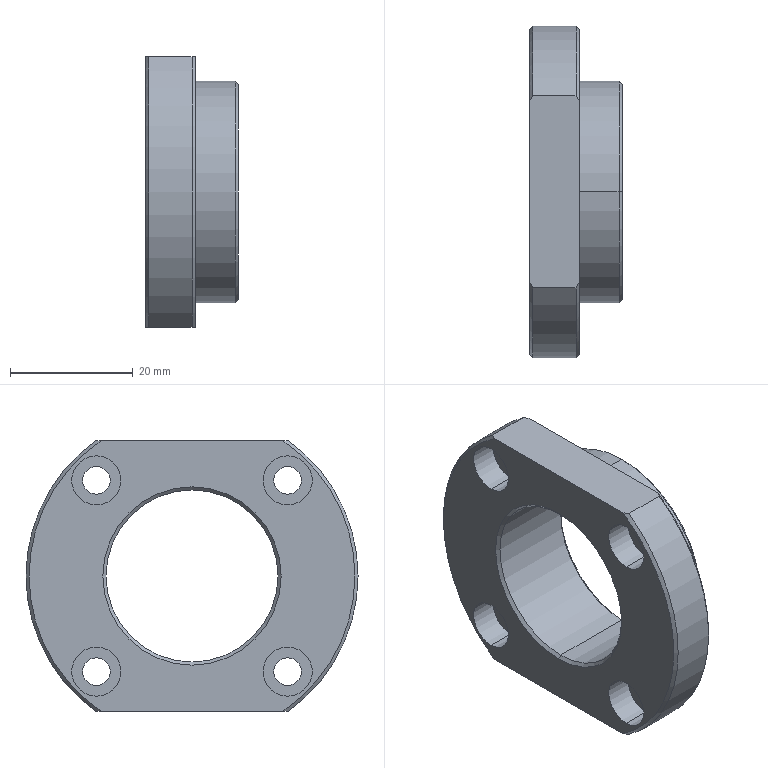Part | SolidWorks | features BaseBody 1 | 1 solid | 41 faces | box 15 x 54 x 44 mm | volume 13318 mm3 | cylinder 22 | cone 10 | plane 9 | commonest cylinder face diameters 4.5 x8 8 x8 28 x2 36 x2 54 x2
STEP:
#1=CARTESIAN_POINT('',(7.,0.,-14.));
#2=VERTEX_POINT('',#1);
#3=CARTESIAN_POINT('',(7.,-14.,0.));
#4=VERTEX_POINT('',#3);
#5=CARTESIAN_POINT('',(7.,0.,0.));
#6=DIRECTION('',(-1.,0.,0.));
#7=DIRECTION('',(0.,0.,1.));
#8=AXIS2_PLACEMENT_3D('',#5,#6,#7);
#9=CIRCLE('',#8,14.);
#10=EDGE_CURVE('',#2,#4,#9,.T.);
#11=ORIENTED_EDGE('',*,*,#10,.F.);
#12=CARTESIAN_POINT('',(-7.,0.,-14.));
#13=VERTEX_POINT('',#12);
#14=CARTESIAN_POINT('',(10.,0.,-14.));
#15=DIRECTION('',(-1.,0.,0.));
#16=VECTOR('',#15,1000.);
#17=LINE('',#14,#16);
#18=EDGE_CURVE('',#2,#13,#17,.T.);
#19=ORIENTED_EDGE('',*,*,#18,.T.);
#20=CARTESIAN_POINT('',(-7.,0.,14.));
#21=VERTEX_POINT('',#20);
#22=CARTESIAN_POINT('',(-7.,0.,0.));
#23=DIRECTION('',(1.,0.,0.));
#24=DIRECTION('',(0.,0.,1.));
#25=AXIS2_PLACEMENT_3D('',#22,#23,#24);
#26=CIRCLE('',#25,14.);
#27=EDGE_CURVE('',#21,#13,#26,.T.);
#28=ORIENTED_EDGE('',*,*,#27,.F.);
#29=CARTESIAN_POINT('',(7.,0.,14.));
#30=VERTEX_POINT('',#29);
#31=CARTESIAN_POINT('',(10.,0.,14.));
#32=DIRECTION('',(-1.,0.,0.));
#33=VECTOR('',#32,1000.);
#34=LINE('',#31,#33);
#35=EDGE_CURVE('',#30,#21,#34,.T.);
#36=ORIENTED_EDGE('',*,*,#35,.F.);
#37=CARTESIAN_POINT('',(7.,0.,0.));
#38=DIRECTION('',(-1.,0.,0.));
#39=DIRECTION('',(0.,0.,1.));
#40=AXIS2_PLACEMENT_3D('',#37,#38,#39);
#41=CIRCLE('',#40,14.);
#42=EDGE_CURVE('',#4,#30,#41,.T.);
#43=ORIENTED_EDGE('',*,*,#42,.F.);
#44=EDGE_LOOP('',(#11,#19,#28,#36,#43));
#45=FACE_OUTER_BOUND('',#44,.T.);
#46=CARTESIAN_POINT('',(10.,0.,0.));
#47=DIRECTION('',(-1.,0.,0.));
#48=DIRECTION('',(0.,0.,1.));
#49=AXIS2_PLACEMENT_3D('',#46,#47,#48);
#50=CYLINDRICAL_SURFACE('',#49,14.);
#51=ADVANCED_FACE('',(#45),#50,.F.);
#52=ORIENTED_EDGE('',*,*,#27,.T.);
#53=CARTESIAN_POINT('',(-7.5,0.,-14.5));
#54=VERTEX_POINT('',#53);
#55=CARTESIAN_POINT('',(-7.5,0.,-14.5));
#56=DIRECTION('',(-0.7071,0.,-0.7071));
#57=VECTOR('',#56,1000.);
#58=LINE('',#55,#57);
#59=EDGE_CURVE('',#13,#54,#58,.T.);
#60=ORIENTED_EDGE('',*,*,#59,.T.);
#61=CARTESIAN_POINT('',(-7.5,0.,14.5));
#62=VERTEX_POINT('',#61);
#63=CARTESIAN_POINT('',(-7.5,0.,0.));
#64=DIRECTION('',(1.,0.,0.));
#65=DIRECTION('',(0.,0.,1.));
#66=AXIS2_PLACEMENT_3D('',#63,#64,#65);
#67=CIRCLE('',#66,14.5);
#68=EDGE_CURVE('',#62,#54,#67,.T.);
#69=ORIENTED_EDGE('',*,*,#68,.F.);
#70=CARTESIAN_POINT('',(-7.5,0.,14.5));
#71=DIRECTION('',(-0.7071,0.,0.7071));
#72=VECTOR('',#71,1000.);
#73=LINE('',#70,#72);
#74=EDGE_CURVE('',#21,#62,#73,.T.);
#75=ORIENTED_EDGE('',*,*,#74,.F.);
#76=EDGE_LOOP('',(#52,#60,#69,#75));
#77=FACE_OUTER_BOUND('',#76,.T.);
#78=CARTESIAN_POINT('',(-7.5,0.,0.));
#79=DIRECTION('',(-1.,0.,0.));
#80=DIRECTION('',(0.,0.,1.));
#81=AXIS2_PLACEMENT_3D('',#78,#79,#80);
#82=CONICAL_SURFACE('',#81,14.5,0.7854);
#83=ADVANCED_FACE('',(#77),#82,.F.);
#84=CARTESIAN_POINT('',(7.,14.,0.));
#85=VERTEX_POINT('',#84);
#86=CARTESIAN_POINT('',(7.,0.,0.));
#87=DIRECTION('',(-1.,0.,0.));
#88=DIRECTION('',(0.,0.,1.));
#89=AXIS2_PLACEMENT_3D('',#86,#87,#88);
#90=CIRCLE('',#89,14.);
#91=EDGE_CURVE('',#85,#2,#90,.T.);
#92=ORIENTED_EDGE('',*,*,#91,.T.);
#93=ORIENTED_EDGE('',*,*,#10,.T.);
#94=CARTESIAN_POINT('',(7.5,-14.5,0.));
#95=VERTEX_POINT('',#94);
#96=CARTESIAN_POINT('',(7.5,-14.5,0.));
#97=DIRECTION('',(0.7071,-0.7071,0.));
#98=VECTOR('',#97,1000.);
#99=LINE('',#96,#98);
#100=EDGE_CURVE('',#4,#95,#99,.T.);
#101=ORIENTED_EDGE('',*,*,#100,.T.);
#102=CARTESIAN_POINT('',(7.5,14.5,0.));
#103=VERTEX_POINT('',#102);
#104=CARTESIAN_POINT('',(7.5,0.,0.));
#105=DIRECTION('',(-1.,0.,0.));
#106=DIRECTION('',(0.,1.,0.));
#107=AXIS2_PLACEMENT_3D('',#104,#105,#106);
#108=CIRCLE('',#107,14.5);
#109=EDGE_CURVE('',#103,#95,#108,.T.);
#110=ORIENTED_EDGE('',*,*,#109,.F.);
#111=CARTESIAN_POINT('',(7.5,14.5,0.));
#112=DIRECTION('',(0.7071,0.7071,0.));
#113=VECTOR('',#112,1000.);
#114=LINE('',#111,#113);
#115=EDGE_CURVE('',#85,#103,#114,.T.);
#116=ORIENTED_EDGE('',*,*,#115,.F.);
#117=EDGE_LOOP('',(#92,#93,#101,#110,#116));
#118=FACE_OUTER_BOUND('',#117,.T.);
#119=CARTESIAN_POINT('',(7.5,0.,0.));
#120=DIRECTION('',(1.,0.,0.));
#121=DIRECTION('',(0.,1.,0.));
#122=AXIS2_PLACEMENT_3D('',#119,#120,#121);
#123=CONICAL_SURFACE('',#122,14.5,0.7854);
#124=ADVANCED_FACE('',(#118),#123,.F.);
#125=CARTESIAN_POINT('',(-3.,15.556,11.556));
#126=VERTEX_POINT('',#125);
#127=CARTESIAN_POINT('',(-3.,15.556,19.556));
#128=VERTEX_POINT('',#127);
#129=CARTESIAN_POINT('',(-3.,15.556,15.556));
#130=DIRECTION('',(-1.,0.,0.));
#131=DIRECTION('',(0.,0.,1.));
#132=AXIS2_PLACEMENT_3D('',#129,#130,#131);
#133=CIRCLE('',#132,4.);
#134=EDGE_CURVE('',#126,#128,#133,.T.);
#135=ORIENTED_EDGE('',*,*,#134,.F.);
#136=CARTESIAN_POINT('',(-7.5,15.556,11.556));
#137=VERTEX_POINT('',#136);
#138=CARTESIAN_POINT('',(0.5,15.556,11.556));
#139=DIRECTION('',(-1.,0.,0.));
#140=VECTOR('',#139,1000.);
#141=LINE('',#138,#140);
#142=EDGE_CURVE('',#126,#137,#141,.T.);
#143=ORIENTED_EDGE('',*,*,#142,.T.);
#144=CARTESIAN_POINT('',(-7.5,15.556,19.556));
#145=VERTEX_POINT('',#144);
#146=CARTESIAN_POINT('',(-7.5,15.556,15.556));
#147=DIRECTION('',(1.,0.,0.));
#148=DIRECTION('',(0.,0.,1.));
#149=AXIS2_PLACEMENT_3D('',#146,#147,#148);
#150=CIRCLE('',#149,4.);
#151=EDGE_CURVE('',#145,#137,#150,.T.);
#152=ORIENTED_EDGE('',*,*,#151,.F.);
#153=CARTESIAN_POINT('',(0.5,15.556,19.556));
#154=DIRECTION('',(-1.,0.,0.));
#155=VECTOR('',#154,1000.);
#156=LINE('',#153,#155);
#157=EDGE_CURVE('',#128,#145,#156,.T.);
#158=ORIENTED_EDGE('',*,*,#157,.F.);
#159=EDGE_LOOP('',(#135,#143,#152,#158));
#160=FACE_OUTER_BOUND('',#159,.T.);
#161=CARTESIAN_POINT('',(0.5,15.556,15.556));
#162=DIRECTION('',(-1.,0.,0.));
#163=DIRECTION('',(0.,0.,1.));
#164=AXIS2_PLACEMENT_3D('',#161,#162,#163);
#165=CYLINDRICAL_SURFACE('',#164,4.);
#166=ADVANCED_FACE('',(#160),#165,.F.);
#167=CARTESIAN_POINT('',(-3.,-15.556,11.556));
#168=VERTEX_POINT('',#167);
#169=CARTESIAN_POINT('',(-3.,-15.556,19.556));
#170=VERTEX_POINT('',#169);
#171=CARTESIAN_POINT('',(-3.,-15.556,15.556));
#172=DIRECTION('',(-1.,0.,0.));
#173=DIRECTION('',(0.,0.,1.));
#174=AXIS2_PLACEMENT_3D('',#171,#172,#173);
#175=CIRCLE('',#174,4.);
#176=EDGE_CURVE('',#168,#170,#175,.T.);
#177=ORIENTED_EDGE('',*,*,#176,.F.);
#178=CARTESIAN_POINT('',(-7.5,-15.556,11.556));
#179=VERTEX_POINT('',#178);
#180=CARTESIAN_POINT('',(0.5,-15.556,11.556));
#181=DIRECTION('',(-1.,0.,0.));
#182=VECTOR('',#181,1000.);
#183=LINE('',#180,#182);
#184=EDGE_CURVE('',#168,#179,#183,.T.);
#185=ORIENTED_EDGE('',*,*,#184,.T.);
#186=CARTESIAN_POINT('',(-7.5,-15.556,19.556));
#187=VERTEX_POINT('',#186);
#188=CARTESIAN_POINT('',(-7.5,-15.556,15.556));
#189=DIRECTION('',(1.,0.,0.));
#190=DIRECTION('',(0.,0.,1.));
#191=AXIS2_PLACEMENT_3D('',#188,#189,#190);
#192=CIRCLE('',#191,4.);
#193=EDGE_CURVE('',#187,#179,#192,.T.);
#194=ORIENTED_EDGE('',*,*,#193,.F.);
#195=CARTESIAN_POINT('',(0.5,-15.556,19.556));
#196=DIRECTION('',(-1.,0.,0.));
#197=VECTOR('',#196,1000.);
#198=LINE('',#195,#197);
#199=EDGE_CURVE('',#170,#187,#198,.T.);
#200=ORIENTED_EDGE('',*,*,#199,.F.);
#201=EDGE_LOOP('',(#177,#185,#194,#200));
#202=FACE_OUTER_BOUND('',#201,.T.);
#203=CARTESIAN_POINT('',(0.5,-15.556,15.556));
#204=DIRECTION('',(-1.,0.,0.));
#205=DIRECTION('',(0.,0.,1.));
#206=AXIS2_PLACEMENT_3D('',#203,#204,#205);
#207=CYLINDRICAL_SURFACE('',#206,4.);
#208=ADVANCED_FACE('',(#202),#207,.F.);
#209=CARTESIAN_POINT('',(-3.,-15.556,-19.556));
#210=VERTEX_POINT('',#209);
#211=CARTESIAN_POINT('',(-3.,-15.556,-11.556));
#212=VERTEX_POINT('',#211);
#213=CARTESIAN_POINT('',(-3.,-15.556,-15.556));
#214=DIRECTION('',(-1.,0.,0.));
#215=DIRECTION('',(0.,0.,1.));
#216=AXIS2_PLACEMENT_3D('',#213,#214,#215);
#217=CIRCLE('',#216,4.);
#218=EDGE_CURVE('',#210,#212,#217,.T.);
#219=ORIENTED_EDGE('',*,*,#218,.F.);
#220=CARTESIAN_POINT('',(-7.5,-15.556,-19.556));
#221=VERTEX_POINT('',#220);
#222=CARTESIAN_POINT('',(0.5,-15.556,-19.556));
#223=DIRECTION('',(-1.,0.,0.));
#224=VECTOR('',#223,1000.);
#225=LINE('',#222,#224);
#226=EDGE_CURVE('',#210,#221,#225,.T.);
#227=ORIENTED_EDGE('',*,*,#226,.T.);
#228=CARTESIAN_POINT('',(-7.5,-15.556,-11.556));
#229=VERTEX_POINT('',#228);
#230=CARTESIAN_POINT('',(-7.5,-15.556,-15.556));
#231=DIRECTION('',(1.,0.,0.));
#232=DIRECTION('',(0.,0.,1.));
#233=AXIS2_PLACEMENT_3D('',#230,#231,#232);
#234=CIRCLE('',#233,4.);
#235=EDGE_CURVE('',#229,#221,#234,.T.);
#236=ORIENTED_EDGE('',*,*,#235,.F.);
#237=CARTESIAN_POINT('',(0.5,-15.556,-11.556));
#238=DIRECTION('',(-1.,0.,0.));
#239=VECTOR('',#238,1000.);
#240=LINE('',#237,#239);
#241=EDGE_CURVE('',#212,#229,#240,.T.);
#242=ORIENTED_EDGE('',*,*,#241,.F.);
#243=EDGE_LOOP('',(#219,#227,#236,#242));
#244=FACE_OUTER_BOUND('',#243,.T.);
#245=CARTESIAN_POINT('',(0.5,-15.556,-15.556));
#246=DIRECTION('',(-1.,0.,0.));
#247=DIRECTION('',(0.,0.,1.));
#248=AXIS2_PLACEMENT_3D('',#245,#246,#247);
#249=CYLINDRICAL_SURFACE('',#248,4.);
#250=ADVANCED_FACE('',(#244),#249,.F.);
#251=CARTESIAN_POINT('',(-3.,15.556,-19.556));
#252=VERTEX_POINT('',#251);
#253=CARTESIAN_POINT('',(-3.,15.556,-11.556));
#254=VERTEX_POINT('',#253);
#255=CARTESIAN_POINT('',(-3.,15.556,-15.556));
#256=DIRECTION('',(-1.,0.,0.));
#257=DIRECTION('',(0.,0.,1.));
#258=AXIS2_PLACEMENT_3D('',#255,#256,#257);
#259=CIRCLE('',#258,4.);
#260=EDGE_CURVE('',#252,#254,#259,.T.);
#261=ORIENTED_EDGE('',*,*,#260,.F.);
#262=CARTESIAN_POINT('',(-7.5,15.556,-19.556));
#263=VERTEX_POINT('',#262);
#264=CARTESIAN_POINT('',(0.5,15.556,-19.556));
#265=DIRECTION('',(-1.,0.,0.));
#266=VECTOR('',#265,1000.);
#267=LINE('',#264,#266);
#268=EDGE_CURVE('',#252,#263,#267,.T.);
#269=ORIENTED_EDGE('',*,*,#268,.T.);
#270=CARTESIAN_POINT('',(-7.5,15.556,-11.556));
#271=VERTEX_POINT('',#270);
#272=CARTESIAN_POINT('',(-7.5,15.556,-15.556));
#273=DIRECTION('',(1.,0.,0.));
#274=DIRECTION('',(0.,0.,1.));
#275=AXIS2_PLACEMENT_3D('',#272,#273,#274);
#276=CIRCLE('',#275,4.);
#277=EDGE_CURVE('',#271,#263,#276,.T.);
#278=ORIENTED_EDGE('',*,*,#277,.F.);
#279=CARTESIAN_POINT('',(0.5,15.556,-11.556));
#280=DIRECTION('',(-1.,0.,0.));
#281=VECTOR('',#280,1000.);
#282=LINE('',#279,#281);
#283=EDGE_CURVE('',#254,#271,#282,.T.);
#284=ORIENTED_EDGE('',*,*,#283,.F.);
#285=EDGE_LOOP('',(#261,#269,#278,#284));
#286=FACE_OUTER_BOUND('',#285,.T.);
#287=CARTESIAN_POINT('',(0.5,15.556,-15.556));
#288=DIRECTION('',(-1.,0.,0.));
#289=DIRECTION('',(0.,0.,1.));
#290=AXIS2_PLACEMENT_3D('',#287,#288,#289);
#291=CYLINDRICAL_SURFACE('',#290,4.);
#292=ADVANCED_FACE('',(#286),#291,.F.);
#293=CARTESIAN_POINT('',(7.5,0.,-17.5));
#294=VERTEX_POINT('',#293);
#295=CARTESIAN_POINT('',(7.5,0.,17.5));
#296=VERTEX_POINT('',#295);
#297=CARTESIAN_POINT('',(7.5,0.,0.));
#298=DIRECTION('',(1.,0.,0.));
#299=DIRECTION('',(0.,0.,1.));
#300=AXIS2_PLACEMENT_3D('',#297,#298,#299);
#301=CIRCLE('',#300,17.5);
#302=EDGE_CURVE('',#294,#296,#301,.T.);
#303=ORIENTED_EDGE('',*,*,#302,.F.);
#304=CARTESIAN_POINT('',(7.,0.,-18.));
#305=VERTEX_POINT('',#304);
#306=CARTESIAN_POINT('',(7.,0.,-18.));
#307=DIRECTION('',(-0.7071,0.,-0.7071));
#308=VECTOR('',#307,1000.);
#309=LINE('',#306,#308);
#310=EDGE_CURVE('',#294,#305,#309,.T.);
#311=ORIENTED_EDGE('',*,*,#310,.T.);
#312=CARTESIAN_POINT('',(7.,0.,18.));
#313=VERTEX_POINT('',#312);
#314=CARTESIAN_POINT('',(7.,0.,0.));
#315=DIRECTION('',(1.,0.,0.));
#316=DIRECTION('',(0.,0.,1.));
#317=AXIS2_PLACEMENT_3D('',#314,#315,#316);
#318=CIRCLE('',#317,18.);
#319=EDGE_CURVE('',#305,#313,#318,.T.);
#320=ORIENTED_EDGE('',*,*,#319,.T.);
#321=CARTESIAN_POINT('',(7.,0.,18.));
#322=DIRECTION('',(-0.7071,0.,0.7071));
#323=VECTOR('',#322,1000.);
#324=LINE('',#321,#323);
#325=EDGE_CURVE('',#296,#313,#324,.T.);
#326=ORIENTED_EDGE('',*,*,#325,.F.);
#327=EDGE_LOOP('',(#303,#311,#320,#326));
#328=FACE_OUTER_BOUND('',#327,.T.);
#329=CARTESIAN_POINT('',(7.,0.,0.));
#330=DIRECTION('',(-1.,0.,0.));
#331=DIRECTION('',(0.,0.,1.));
#332=AXIS2_PLACEMENT_3D('',#329,#330,#331);
#333=CONICAL_SURFACE('',#332,18.,0.7854);
#334=ADVANCED_FACE('',(#328),#333,.T.);
#335=ORIENTED_EDGE('',*,*,#319,.F.);
#336=CARTESIAN_POINT('',(0.5,0.,-18.));
#337=VERTEX_POINT('',#336);
#338=CARTESIAN_POINT('',(10.,0.,-18.));
#339=DIRECTION('',(-1.,0.,0.));
#340=VECTOR('',#339,1000.);
#341=LINE('',#338,#340);
#342=EDGE_CURVE('',#305,#337,#341,.T.);
#343=ORIENTED_EDGE('',*,*,#342,.T.);
#344=CARTESIAN_POINT('',(0.5,0.,18.));
#345=VERTEX_POINT('',#344);
#346=CARTESIAN_POINT('',(0.5,0.,0.));
#347=DIRECTION('',(-1.,0.,0.));
#348=DIRECTION('',(0.,0.,1.));
#349=AXIS2_PLACEMENT_3D('',#346,#347,#348);
#350=CIRCLE('',#349,18.);
#351=EDGE_CURVE('',#345,#337,#350,.T.);
#352=ORIENTED_EDGE('',*,*,#351,.F.);
#353=CARTESIAN_POINT('',(10.,0.,18.));
#354=DIRECTION('',(-1.,0.,0.));
#355=VECTOR('',#354,1000.);
#356=LINE('',#353,#355);
#357=EDGE_CURVE('',#313,#345,#356,.T.);
#358=ORIENTED_EDGE('',*,*,#357,.F.);
#359=EDGE_LOOP('',(#335,#343,#352,#358));
#360=FACE_OUTER_BOUND('',#359,.T.);
#361=CARTESIAN_POINT('',(10.,0.,0.));
#362=DIRECTION('',(-1.,0.,0.));
#363=DIRECTION('',(0.,0.,1.));
#364=AXIS2_PLACEMENT_3D('',#361,#362,#363);
#365=CYLINDRICAL_SURFACE('',#364,18.);
#366=ADVANCED_FACE('',(#360),#365,.T.);
#367=CARTESIAN_POINT('',(0.5,15.556,13.306));
#368=VERTEX_POINT('',#367);
#369=CARTESIAN_POINT('',(0.5,15.556,17.806));
#370=VERTEX_POINT('',#369);
#371=CARTESIAN_POINT('',(0.5,15.556,15.556));
#372=DIRECTION('',(-1.,0.,0.));
#373=DIRECTION('',(0.,0.,1.));
#374=AXIS2_PLACEMENT_3D('',#371,#372,#373);
#375=CIRCLE('',#374,2.25);
#376=EDGE_CURVE('',#368,#370,#375,.T.);
#377=ORIENTED_EDGE('',*,*,#376,.F.);
#378=CARTESIAN_POINT('',(-3.,15.556,13.306));
#379=VERTEX_POINT('',#378);
#380=CARTESIAN_POINT('',(0.5,15.556,13.306));
#381=DIRECTION('',(-1.,0.,0.));
#382=VECTOR('',#381,1000.);
#383=LINE('',#380,#382);
#384=EDGE_CURVE('',#368,#379,#383,.T.);
#385=ORIENTED_EDGE('',*,*,#384,.T.);
#386=CARTESIAN_POINT('',(-3.,15.556,17.806));
#387=VERTEX_POINT('',#386);
#388=CARTESIAN_POINT('',(-3.,15.556,15.556));
#389=DIRECTION('',(1.,0.,0.));
#390=DIRECTION('',(0.,0.,1.));
#391=AXIS2_PLACEMENT_3D('',#388,#389,#390);
#392=CIRCLE('',#391,2.25);
#393=EDGE_CURVE('',#387,#379,#392,.T.);
#394=ORIENTED_EDGE('',*,*,#393,.F.);
#395=CARTESIAN_POINT('',(0.5,15.556,17.806));
#396=DIRECTION('',(-1.,0.,0.));
#397=VECTOR('',#396,1000.);
#398=LINE('',#395,#397);
#399=EDGE_CURVE('',#370,#387,#398,.T.);
#400=ORIENTED_EDGE('',*,*,#399,.F.);
#401=EDGE_LOOP('',(#377,#385,#394,#400));
#402=FACE_OUTER_BOUND('',#401,.T.);
#403=CARTESIAN_POINT('',(0.5,15.556,15.556));
#404=DIRECTION('',(-1.,0.,0.));
#405=DIRECTION('',(0.,0.,1.));
#406=AXIS2_PLACEMENT_3D('',#403,#404,#405);
#407=CYLINDRICAL_SURFACE('',#406,2.25);
#408=ADVANCED_FACE('',(#402),#407,.F.);
#409=CARTESIAN_POINT('',(0.5,-15.556,13.306));
#410=VERTEX_POINT('',#409);
#411=CARTESIAN_POINT('',(0.5,-15.556,17.806));
#412=VERTEX_POINT('',#411);
#413=CARTESIAN_POINT('',(0.5,-15.556,15.556));
#414=DIRECTION('',(-1.,0.,0.));
#415=DIRECTION('',(0.,0.,1.));
#416=AXIS2_PLACEMENT_3D('',#413,#414,#415);
#417=CIRCLE('',#416,2.25);
#418=EDGE_CURVE('',#410,#412,#417,.T.);
#419=ORIENTED_EDGE('',*,*,#418,.F.);
#420=CARTESIAN_POINT('',(-3.,-15.556,13.306));
#421=VERTEX_POINT('',#420);
#422=CARTESIAN_POINT('',(0.5,-15.556,13.306));
#423=DIRECTION('',(-1.,0.,0.));
#424=VECTOR('',#423,1000.);
#425=LINE('',#422,#424);
#426=EDGE_CURVE('',#410,#421,#425,.T.);
#427=ORIENTED_EDGE('',*,*,#426,.T.);
#428=CARTESIAN_POINT('',(-3.,-15.556,17.806));
#429=VERTEX_POINT('',#428);
#430=CARTESIAN_POINT('',(-3.,-15.556,15.556));
#431=DIRECTION('',(1.,0.,0.));
#432=DIRECTION('',(0.,0.,1.));
#433=AXIS2_PLACEMENT_3D('',#430,#431,#432);
#434=CIRCLE('',#433,2.25);
#435=EDGE_CURVE('',#429,#421,#434,.T.);
#436=ORIENTED_EDGE('',*,*,#435,.F.);
#437=CARTESIAN_POINT('',(0.5,-15.556,17.806));
#438=DIRECTION('',(-1.,0.,0.));
#439=VECTOR('',#438,1000.);
#440=LINE('',#437,#439);
#441=EDGE_CURVE('',#412,#429,#440,.T.);
#442=ORIENTED_EDGE('',*,*,#441,.F.);
#443=EDGE_LOOP('',(#419,#427,#436,#442));
#444=FACE_OUTER_BOUND('',#443,.T.);
#445=CARTESIAN_POINT('',(0.5,-15.556,15.556));
#446=DIRECTION('',(-1.,0.,0.));
#447=DIRECTION('',(0.,0.,1.));
#448=AXIS2_PLACEMENT_3D('',#445,#446,#447);
#449=CYLINDRICAL_SURFACE('',#448,2.25);
#450=ADVANCED_FACE('',(#444),#449,.F.);
#451=CARTESIAN_POINT('',(0.5,-15.556,-17.806));
#452=VERTEX_POINT('',#451);
#453=CARTESIAN_POINT('',(0.5,-15.556,-13.306));
#454=VERTEX_POINT('',#453);
#455=CARTESIAN_POINT('',(0.5,-15.556,-15.556));
#456=DIRECTION('',(-1.,0.,0.));
#457=DIRECTION('',(0.,0.,1.));
#458=AXIS2_PLACEMENT_3D('',#455,#456,#457);
#459=CIRCLE('',#458,2.25);
#460=EDGE_CURVE('',#452,#454,#459,.T.);
#461=ORIENTED_EDGE('',*,*,#460,.F.);
#462=CARTESIAN_POINT('',(-3.,-15.556,-17.806));
#463=VERTEX_POINT('',#462);
#464=CARTESIAN_POINT('',(0.5,-15.556,-17.806));
#465=DIRECTION('',(-1.,0.,0.));
#466=VECTOR('',#465,1000.);
#467=LINE('',#464,#466);
#468=EDGE_CURVE('',#452,#463,#467,.T.);
#469=ORIENTED_EDGE('',*,*,#468,.T.);
#470=CARTESIAN_POINT('',(-3.,-15.556,-13.306));
#471=VERTEX_POINT('',#470);
#472=CARTESIAN_POINT('',(-3.,-15.556,-15.556));
#473=DIRECTION('',(1.,0.,0.));
#474=DIRECTION('',(0.,0.,1.));
#475=AXIS2_PLACEMENT_3D('',#472,#473,#474);
#476=CIRCLE('',#475,2.25);
#477=EDGE_CURVE('',#471,#463,#476,.T.);
#478=ORIENTED_EDGE('',*,*,#477,.F.);
#479=CARTESIAN_POINT('',(0.5,-15.556,-13.306));
#480=DIRECTION('',(-1.,0.,0.));
#481=VECTOR('',#480,1000.);
#482=LINE('',#479,#481);
#483=EDGE_CURVE('',#454,#471,#482,.T.);
#484=ORIENTED_EDGE('',*,*,#483,.F.);
#485=EDGE_LOOP('',(#461,#469,#478,#484));
#486=FACE_OUTER_BOUND('',#485,.T.);
#487=CARTESIAN_POINT('',(0.5,-15.556,-15.556));
#488=DIRECTION('',(-1.,0.,0.));
#489=DIRECTION('',(0.,0.,1.));
#490=AXIS2_PLACEMENT_3D('',#487,#488,#489);
#491=CYLINDRICAL_SURFACE('',#490,2.25);
#492=ADVANCED_FACE('',(#486),#491,.F.);
#493=CARTESIAN_POINT('',(0.5,15.556,-17.806));
#494=VERTEX_POINT('',#493);
#495=CARTESIAN_POINT('',(0.5,15.556,-13.306));
#496=VERTEX_POINT('',#495);
#497=CARTESIAN_POINT('',(0.5,15.556,-15.556));
#498=DIRECTION('',(-1.,0.,0.));
#499=DIRECTION('',(0.,0.,1.));
#500=AXIS2_PLACEMENT_3D('',#497,#498,#499);
#501=CIRCLE('',#500,2.25);
#502=EDGE_CURVE('',#494,#496,#501,.T.);
#503=ORIENTED_EDGE('',*,*,#502,.F.);
#504=CARTESIAN_POINT('',(-3.,15.556,-17.806));
#505=VERTEX_POINT('',#504);
#506=CARTESIAN_POINT('',(0.5,15.556,-17.806));
#507=DIRECTION('',(-1.,0.,0.));
#508=VECTOR('',#507,1000.);
#509=LINE('',#506,#508);
#510=EDGE_CURVE('',#494,#505,#509,.T.);
#511=ORIENTED_EDGE('',*,*,#510,.T.);
#512=CARTESIAN_POINT('',(-3.,15.556,-13.306));
#513=VERTEX_POINT('',#512);
#514=CARTESIAN_POINT('',(-3.,15.556,-15.556));
#515=DIRECTION('',(1.,0.,0.));
#516=DIRECTION('',(0.,0.,1.));
#517=AXIS2_PLACEMENT_3D('',#514,#515,#516);
#518=CIRCLE('',#517,2.25);
#519=EDGE_CURVE('',#513,#505,#518,.T.);
#520=ORIENTED_EDGE('',*,*,#519,.F.);
#521=CARTESIAN_POINT('',(0.5,15.556,-13.306));
#522=DIRECTION('',(-1.,0.,0.));
#523=VECTOR('',#522,1000.);
#524=LINE('',#521,#523);
#525=EDGE_CURVE('',#496,#513,#524,.T.);
#526=ORIENTED_EDGE('',*,*,#525,.F.);
#527=EDGE_LOOP('',(#503,#511,#520,#526));
#528=FACE_OUTER_BOUND('',#527,.T.);
#529=CARTESIAN_POINT('',(0.5,15.556,-15.556));
#530=DIRECTION('',(-1.,0.,0.));
#531=DIRECTION('',(0.,0.,1.));
#532=AXIS2_PLACEMENT_3D('',#529,#530,#531);
#533=CYLINDRICAL_SURFACE('',#532,2.25);
#534=ADVANCED_FACE('',(#528),#533,.F.);
#535=ORIENTED_EDGE('',*,*,#18,.F.);
#536=ORIENTED_EDGE('',*,*,#91,.F.);
#537=CARTESIAN_POINT('',(7.,0.,0.));
#538=DIRECTION('',(-1.,0.,0.));
#539=DIRECTION('',(0.,0.,1.));
#540=AXIS2_PLACEMENT_3D('',#537,#538,#539);
#541=CIRCLE('',#540,14.);
#542=EDGE_CURVE('',#30,#85,#541,.T.);
#543=ORIENTED_EDGE('',*,*,#542,.F.);
#544=ORIENTED_EDGE('',*,*,#35,.T.);
#545=CARTESIAN_POINT('',(-7.,0.,0.));
#546=DIRECTION('',(1.,0.,0.));
#547=DIRECTION('',(0.,0.,1.));
#548=AXIS2_PLACEMENT_3D('',#545,#546,#547);
#549=CIRCLE('',#548,14.);
#550=EDGE_CURVE('',#13,#21,#549,.T.);
#551=ORIENTED_EDGE('',*,*,#550,.F.);
#552=EDGE_LOOP('',(#535,#536,#543,#544,#551));
#553=FACE_OUTER_BOUND('',#552,.T.);
#554=CARTESIAN_POINT('',(10.,0.,0.));
#555=DIRECTION('',(-1.,0.,0.));
#556=DIRECTION('',(0.,0.,1.));
#557=AXIS2_PLACEMENT_3D('',#554,#555,#556);
#558=CYLINDRICAL_SURFACE('',#557,14.);
#559=ADVANCED_FACE('',(#553),#558,.F.);
#560=ORIENTED_EDGE('',*,*,#59,.F.);
#561=ORIENTED_EDGE('',*,*,#550,.T.);
#562=ORIENTED_EDGE('',*,*,#74,.T.);
#563=CARTESIAN_POINT('',(-7.5,0.,0.));
#564=DIRECTION('',(1.,0.,0.));
#565=DIRECTION('',(0.,0.,1.));
#566=AXIS2_PLACEMENT_3D('',#563,#564,#565);
#567=CIRCLE('',#566,14.5);
#568=EDGE_CURVE('',#54,#62,#567,.T.);
#569=ORIENTED_EDGE('',*,*,#568,.F.);
#570=EDGE_LOOP('',(#560,#561,#562,#569));
#571=FACE_OUTER_BOUND('',#570,.T.);
#572=CARTESIAN_POINT('',(-7.5,0.,0.));
#573=DIRECTION('',(-1.,0.,0.));
#574=DIRECTION('',(0.,0.,1.));
#575=AXIS2_PLACEMENT_3D('',#572,#573,#574);
#576=CONICAL_SURFACE('',#575,14.5,0.7854);
#577=ADVANCED_FACE('',(#571),#576,.F.);
#578=ORIENTED_EDGE('',*,*,#100,.F.);
#579=ORIENTED_EDGE('',*,*,#42,.T.);
#580=ORIENTED_EDGE('',*,*,#542,.T.);
#581=ORIENTED_EDGE('',*,*,#115,.T.);
#582=CARTESIAN_POINT('',(7.5,0.,0.));
#583=DIRECTION('',(-1.,0.,0.));
#584=DIRECTION('',(0.,1.,0.));
#585=AXIS2_PLACEMENT_3D('',#582,#583,#584);
#586=CIRCLE('',#585,14.5);
#587=EDGE_CURVE('',#95,#103,#586,.T.);
#588=ORIENTED_EDGE('',*,*,#587,.F.);
#589=EDGE_LOOP('',(#578,#579,#580,#581,#588));
#590=FACE_OUTER_BOUND('',#589,.T.);
#591=CARTESIAN_POINT('',(7.5,0.,0.));
#592=DIRECTION('',(1.,0.,0.));
#593=DIRECTION('',(0.,1.,0.));
#594=AXIS2_PLACEMENT_3D('',#591,#592,#593);
#595=CONICAL_SURFACE('',#594,14.5,0.7854);
#596=ADVANCED_FACE('',(#590),#595,.F.);
#597=ORIENTED_EDGE('',*,*,#151,.T.);
#598=CARTESIAN_POINT('',(-7.5,15.556,15.556));
#599=DIRECTION('',(1.,0.,0.));
#600=DIRECTION('',(0.,0.,1.));
#601=AXIS2_PLACEMENT_3D('',#598,#599,#600);
#602=CIRCLE('',#601,4.);
#603=EDGE_CURVE('',#137,#145,#602,.T.);
#604=ORIENTED_EDGE('',*,*,#603,.T.);
#605=EDGE_LOOP('',(#597,#604));
#606=FACE_BOUND('',#605,.T.);
#607=ORIENTED_EDGE('',*,*,#193,.T.);
#608=CARTESIAN_POINT('',(-7.5,-15.556,15.556));
#609=DIRECTION('',(1.,0.,0.));
#610=DIRECTION('',(0.,0.,1.));
#611=AXIS2_PLACEMENT_3D('',#608,#609,#610);
#612=CIRCLE('',#611,4.);
#613=EDGE_CURVE('',#179,#187,#612,.T.);
#614=ORIENTED_EDGE('',*,*,#613,.T.);
#615=EDGE_LOOP('',(#607,#614));
#616=FACE_BOUND('',#615,.T.);
#617=ORIENTED_EDGE('',*,*,#235,.T.);
#618=CARTESIAN_POINT('',(-7.5,-15.556,-15.556));
#619=DIRECTION('',(1.,0.,0.));
#620=DIRECTION('',(0.,0.,1.));
#621=AXIS2_PLACEMENT_3D('',#618,#619,#620);
#622=CIRCLE('',#621,4.);
#623=EDGE_CURVE('',#221,#229,#622,.T.);
#624=ORIENTED_EDGE('',*,*,#623,.T.);
#625=EDGE_LOOP('',(#617,#624));
#626=FACE_BOUND('',#625,.T.);
#627=ORIENTED_EDGE('',*,*,#277,.T.);
#628=CARTESIAN_POINT('',(-7.5,15.556,-15.556));
#629=DIRECTION('',(1.,0.,0.));
#630=DIRECTION('',(0.,0.,1.));
#631=AXIS2_PLACEMENT_3D('',#628,#629,#630);
#632=CIRCLE('',#631,4.);
#633=EDGE_CURVE('',#263,#271,#632,.T.);
#634=ORIENTED_EDGE('',*,*,#633,.T.);
#635=EDGE_LOOP('',(#627,#634));
#636=FACE_BOUND('',#635,.T.);
#637=CARTESIAN_POINT('',(-7.5,-14.773,22.));
#638=VERTEX_POINT('',#637);
#639=CARTESIAN_POINT('',(-7.5,14.773,22.));
#640=VERTEX_POINT('',#639);
#641=CARTESIAN_POINT('',(-7.5,26.5,22.));
#642=DIRECTION('',(0.,1.,0.));
#643=VECTOR('',#642,1000.);
#644=LINE('',#641,#643);
#645=EDGE_CURVE('',#638,#640,#644,.T.);
#646=ORIENTED_EDGE('',*,*,#645,.T.);
#647=CARTESIAN_POINT('',(-7.5,14.773,-22.));
#648=VERTEX_POINT('',#647);
#649=CARTESIAN_POINT('',(-7.5,0.,0.));
#650=DIRECTION('',(-1.,0.,0.));
#651=DIRECTION('',(0.,0.,-1.));
#652=AXIS2_PLACEMENT_3D('',#649,#650,#651);
#653=CIRCLE('',#652,26.5);
#654=EDGE_CURVE('',#640,#648,#653,.T.);
#655=ORIENTED_EDGE('',*,*,#654,.T.);
#656=CARTESIAN_POINT('',(-7.5,-14.773,-22.));
#657=VERTEX_POINT('',#656);
#658=CARTESIAN_POINT('',(-7.5,26.5,-22.));
#659=DIRECTION('',(0.,-1.,0.));
#660=VECTOR('',#659,1000.);
#661=LINE('',#658,#660);
#662=EDGE_CURVE('',#648,#657,#661,.T.);
#663=ORIENTED_EDGE('',*,*,#662,.T.);
#664=CARTESIAN_POINT('',(-7.5,0.,0.));
#665=DIRECTION('',(-1.,0.,0.));
#666=DIRECTION('',(0.,0.,-1.));
#667=AXIS2_PLACEMENT_3D('',#664,#665,#666);
#668=CIRCLE('',#667,26.5);
#669=EDGE_CURVE('',#657,#638,#668,.T.);
#670=ORIENTED_EDGE('',*,*,#669,.T.);
#671=EDGE_LOOP('',(#646,#655,#663,#670));
#672=FACE_OUTER_BOUND('',#671,.T.);
#673=ORIENTED_EDGE('',*,*,#68,.T.);
#674=ORIENTED_EDGE('',*,*,#568,.T.);
#675=EDGE_LOOP('',(#673,#674));
#676=FACE_BOUND('',#675,.T.);
#677=CARTESIAN_POINT('',(-7.5,26.5,0.));
#678=DIRECTION('',(-1.,0.,0.));
#679=DIRECTION('',(0.,0.,1.));
#680=AXIS2_PLACEMENT_3D('',#677,#678,#679);
#681=PLANE('',#680);
#682=ADVANCED_FACE('',(#606,#616,#626,#636,#672,#676),#681,.T.);
#683=ORIENTED_EDGE('',*,*,#109,.T.);
#684=ORIENTED_EDGE('',*,*,#587,.T.);
#685=EDGE_LOOP('',(#683,#684));
#686=FACE_BOUND('',#685,.T.);
#687=CARTESIAN_POINT('',(7.5,0.,0.));
#688=DIRECTION('',(1.,0.,0.));
#689=DIRECTION('',(0.,0.,1.));
#690=AXIS2_PLACEMENT_3D('',#687,#688,#689);
#691=CIRCLE('',#690,17.5);
#692=EDGE_CURVE('',#296,#294,#691,.T.);
#693=ORIENTED_EDGE('',*,*,#692,.T.);
#694=ORIENTED_EDGE('',*,*,#302,.T.);
#695=EDGE_LOOP('',(#693,#694));
#696=FACE_OUTER_BOUND('',#695,.T.);
#697=CARTESIAN_POINT('',(7.5,14.5,0.));
#698=DIRECTION('',(1.,0.,0.));
#699=DIRECTION('',(0.,0.,-1.));
#700=AXIS2_PLACEMENT_3D('',#697,#698,#699);
#701=PLANE('',#700);
#702=ADVANCED_FACE('',(#686,#696),#701,.T.);
#703=ORIENTED_EDGE('',*,*,#142,.F.);
#704=CARTESIAN_POINT('',(-3.,15.556,15.556));
#705=DIRECTION('',(-1.,0.,0.));
#706=DIRECTION('',(0.,0.,1.));
#707=AXIS2_PLACEMENT_3D('',#704,#705,#706);
#708=CIRCLE('',#707,4.);
#709=EDGE_CURVE('',#128,#126,#708,.T.);
#710=ORIENTED_EDGE('',*,*,#709,.F.);
#711=ORIENTED_EDGE('',*,*,#157,.T.);
#712=ORIENTED_EDGE('',*,*,#603,.F.);
#713=EDGE_LOOP('',(#703,#710,#711,#712));
#714=FACE_OUTER_BOUND('',#713,.T.);
#715=CARTESIAN_POINT('',(0.5,15.556,15.556));
#716=DIRECTION('',(-1.,0.,0.));
#717=DIRECTION('',(0.,0.,1.));
#718=AXIS2_PLACEMENT_3D('',#715,#716,#717);
#719=CYLINDRICAL_SURFACE('',#718,4.);
#720=ADVANCED_FACE('',(#714),#719,.F.);
#721=ORIENTED_EDGE('',*,*,#184,.F.);
#722=CARTESIAN_POINT('',(-3.,-15.556,15.556));
#723=DIRECTION('',(-1.,0.,0.));
#724=DIRECTION('',(0.,0.,1.));
#725=AXIS2_PLACEMENT_3D('',#722,#723,#724);
#726=CIRCLE('',#725,4.);
#727=EDGE_CURVE('',#170,#168,#726,.T.);
#728=ORIENTED_EDGE('',*,*,#727,.F.);
#729=ORIENTED_EDGE('',*,*,#199,.T.);
#730=ORIENTED_EDGE('',*,*,#613,.F.);
#731=EDGE_LOOP('',(#721,#728,#729,#730));
#732=FACE_OUTER_BOUND('',#731,.T.);
#733=CARTESIAN_POINT('',(0.5,-15.556,15.556));
#734=DIRECTION('',(-1.,0.,0.));
#735=DIRECTION('',(0.,0.,1.));
#736=AXIS2_PLACEMENT_3D('',#733,#734,#735);
#737=CYLINDRICAL_SURFACE('',#736,4.);
#738=ADVANCED_FACE('',(#732),#737,.F.);
#739=ORIENTED_EDGE('',*,*,#226,.F.);
#740=CARTESIAN_POINT('',(-3.,-15.556,-15.556));
#741=DIRECTION('',(-1.,0.,0.));
#742=DIRECTION('',(0.,0.,1.));
#743=AXIS2_PLACEMENT_3D('',#740,#741,#742);
#744=CIRCLE('',#743,4.);
#745=EDGE_CURVE('',#212,#210,#744,.T.);
#746=ORIENTED_EDGE('',*,*,#745,.F.);
#747=ORIENTED_EDGE('',*,*,#241,.T.);
#748=ORIENTED_EDGE('',*,*,#623,.F.);
#749=EDGE_LOOP('',(#739,#746,#747,#748));
#750=FACE_OUTER_BOUND('',#749,.T.);
#751=CARTESIAN_POINT('',(0.5,-15.556,-15.556));
#752=DIRECTION('',(-1.,0.,0.));
#753=DIRECTION('',(0.,0.,1.));
#754=AXIS2_PLACEMENT_3D('',#751,#752,#753);
#755=CYLINDRICAL_SURFACE('',#754,4.);
#756=ADVANCED_FACE('',(#750),#755,.F.);
#757=ORIENTED_EDGE('',*,*,#268,.F.);
#758=CARTESIAN_POINT('',(-3.,15.556,-15.556));
#759=DIRECTION('',(-1.,0.,0.));
#760=DIRECTION('',(0.,0.,1.));
#761=AXIS2_PLACEMENT_3D('',#758,#759,#760);
#762=CIRCLE('',#761,4.);
#763=EDGE_CURVE('',#254,#252,#762,.T.);
#764=ORIENTED_EDGE('',*,*,#763,.F.);
#765=ORIENTED_EDGE('',*,*,#283,.T.);
#766=ORIENTED_EDGE('',*,*,#633,.F.);
#767=EDGE_LOOP('',(#757,#764,#765,#766));
#768=FACE_OUTER_BOUND('',#767,.T.);
#769=CARTESIAN_POINT('',(0.5,15.556,-15.556));
#770=DIRECTION('',(-1.,0.,0.));
#771=DIRECTION('',(0.,0.,1.));
#772=AXIS2_PLACEMENT_3D('',#769,#770,#771);
#773=CYLINDRICAL_SURFACE('',#772,4.);
#774=ADVANCED_FACE('',(#768),#773,.F.);
#775=CARTESIAN_POINT('',(-7.,15.652,22.));
#776=VERTEX_POINT('',#775);
#777=CARTESIAN_POINT('',(-7.5,14.773,22.));
#778=CARTESIAN_POINT('',(-7.336,15.068,22.));
#779=CARTESIAN_POINT('',(-7.169,15.361,22.));
#780=CARTESIAN_POINT('',(-7.,15.652,22.));
#781=B_SPLINE_CURVE_WITH_KNOTS('',3,(#777,#778,#779,#780),.UNSPECIFIED.,.F.,.F.,(4,4),(0.,0.001011),.UNSPECIFIED.);
#782=EDGE_CURVE('',#640,#776,#781,.T.);
#783=ORIENTED_EDGE('',*,*,#782,.T.);
#784=CARTESIAN_POINT('',(-7.,15.652,-22.));
#785=VERTEX_POINT('',#784);
#786=CARTESIAN_POINT('',(-7.,0.,0.));
#787=DIRECTION('',(-1.,0.,0.));
#788=DIRECTION('',(0.,0.,-1.));
#789=AXIS2_PLACEMENT_3D('',#786,#787,#788);
#790=CIRCLE('',#789,27.);
#791=EDGE_CURVE('',#776,#785,#790,.T.);
#792=ORIENTED_EDGE('',*,*,#791,.T.);
#793=CARTESIAN_POINT('',(-7.,15.652,-22.));
#794=CARTESIAN_POINT('',(-7.169,15.361,-22.));
#795=CARTESIAN_POINT('',(-7.336,15.068,-22.));
#796=CARTESIAN_POINT('',(-7.5,14.773,-22.));
#797=B_SPLINE_CURVE_WITH_KNOTS('',3,(#793,#794,#795,#796),.UNSPECIFIED.,.F.,.F.,(4,4),(0.,0.001011),.UNSPECIFIED.);
#798=EDGE_CURVE('',#785,#648,#797,.T.);
#799=ORIENTED_EDGE('',*,*,#798,.T.);
#800=ORIENTED_EDGE('',*,*,#654,.F.);
#801=EDGE_LOOP('',(#783,#792,#799,#800));
#802=FACE_OUTER_BOUND('',#801,.T.);
#803=CARTESIAN_POINT('',(-7.,0.,0.));
#804=DIRECTION('',(1.,0.,0.));
#805=DIRECTION('',(0.,0.,-1.));
#806=AXIS2_PLACEMENT_3D('',#803,#804,#805);
#807=CONICAL_SURFACE('',#806,27.,0.7854);
#808=ADVANCED_FACE('',(#802),#807,.T.);
#809=CARTESIAN_POINT('',(0.,15.652,22.));
#810=VERTEX_POINT('',#809);
#811=CARTESIAN_POINT('',(0.5,15.652,22.));
#812=DIRECTION('',(1.,0.,0.));
#813=VECTOR('',#812,1000.);
#814=LINE('',#811,#813);
#815=EDGE_CURVE('',#776,#810,#814,.T.);
#816=ORIENTED_EDGE('',*,*,#815,.F.);
#817=ORIENTED_EDGE('',*,*,#782,.F.);
#818=ORIENTED_EDGE('',*,*,#645,.F.);
#819=CARTESIAN_POINT('',(-7.,-15.652,22.));
#820=VERTEX_POINT('',#819);
#821=CARTESIAN_POINT('',(-7.,-15.652,22.));
#822=CARTESIAN_POINT('',(-7.169,-15.361,22.));
#823=CARTESIAN_POINT('',(-7.336,-15.068,22.));
#824=CARTESIAN_POINT('',(-7.5,-14.773,22.));
#825=B_SPLINE_CURVE_WITH_KNOTS('',3,(#821,#822,#823,#824),.UNSPECIFIED.,.F.,.F.,(4,4),(0.,0.001011),.UNSPECIFIED.);
#826=EDGE_CURVE('',#820,#638,#825,.T.);
#827=ORIENTED_EDGE('',*,*,#826,.F.);
#828=CARTESIAN_POINT('',(0.,-15.652,22.));
#829=VERTEX_POINT('',#828);
#830=CARTESIAN_POINT('',(0.5,-15.652,22.));
#831=DIRECTION('',(-1.,0.,0.));
#832=VECTOR('',#831,1000.);
#833=LINE('',#830,#832);
#834=EDGE_CURVE('',#829,#820,#833,.T.);
#835=ORIENTED_EDGE('',*,*,#834,.F.);
#836=CARTESIAN_POINT('',(0.5,-14.773,22.));
#837=VERTEX_POINT('',#836);
#838=CARTESIAN_POINT('',(0.5,-14.773,22.));
#839=CARTESIAN_POINT('',(0.3358,-15.068,22.));
#840=CARTESIAN_POINT('',(0.1691,-15.361,22.));
#841=CARTESIAN_POINT('',(0.,-15.652,22.));
#842=B_SPLINE_CURVE_WITH_KNOTS('',3,(#838,#839,#840,#841),.UNSPECIFIED.,.F.,.F.,(4,4),(0.,0.001011),.UNSPECIFIED.);
#843=EDGE_CURVE('',#837,#829,#842,.T.);
#844=ORIENTED_EDGE('',*,*,#843,.F.);
#845=CARTESIAN_POINT('',(0.5,14.773,22.));
#846=VERTEX_POINT('',#845);
#847=CARTESIAN_POINT('',(0.5,49.,22.));
#848=DIRECTION('',(0.,-1.,0.));
#849=VECTOR('',#848,1000.);
#850=LINE('',#847,#849);
#851=EDGE_CURVE('',#846,#837,#850,.T.);
#852=ORIENTED_EDGE('',*,*,#851,.F.);
#853=CARTESIAN_POINT('',(0.,15.652,22.));
#854=CARTESIAN_POINT('',(0.1691,15.361,22.));
#855=CARTESIAN_POINT('',(0.3358,15.068,22.));
#856=CARTESIAN_POINT('',(0.5,14.773,22.));
#857=B_SPLINE_CURVE_WITH_KNOTS('',3,(#853,#854,#855,#856),.UNSPECIFIED.,.F.,.F.,(4,4),(0.,0.001011),.UNSPECIFIED.);
#858=EDGE_CURVE('',#810,#846,#857,.T.);
#859=ORIENTED_EDGE('',*,*,#858,.F.);
#860=EDGE_LOOP('',(#816,#817,#818,#827,#835,#844,#852,#859));
#861=FACE_OUTER_BOUND('',#860,.T.);
#862=CARTESIAN_POINT('',(0.5,49.,22.));
#863=DIRECTION('',(0.,0.,-1.));
#864=DIRECTION('',(-1.,0.,0.));
#865=AXIS2_PLACEMENT_3D('',#862,#863,#864);
#866=PLANE('',#865);
#867=ADVANCED_FACE('',(#861),#866,.F.);
#868=ORIENTED_EDGE('',*,*,#826,.T.);
#869=ORIENTED_EDGE('',*,*,#669,.F.);
#870=CARTESIAN_POINT('',(-7.,-15.652,-22.));
#871=VERTEX_POINT('',#870);
#872=CARTESIAN_POINT('',(-7.5,-14.773,-22.));
#873=CARTESIAN_POINT('',(-7.336,-15.068,-22.));
#874=CARTESIAN_POINT('',(-7.169,-15.361,-22.));
#875=CARTESIAN_POINT('',(-7.,-15.652,-22.));
#876=B_SPLINE_CURVE_WITH_KNOTS('',3,(#872,#873,#874,#875),.UNSPECIFIED.,.F.,.F.,(4,4),(0.,0.001011),.UNSPECIFIED.);
#877=EDGE_CURVE('',#657,#871,#876,.T.);
#878=ORIENTED_EDGE('',*,*,#877,.T.);
#879=CARTESIAN_POINT('',(-7.,0.,0.));
#880=DIRECTION('',(-1.,0.,0.));
#881=DIRECTION('',(0.,0.,-1.));
#882=AXIS2_PLACEMENT_3D('',#879,#880,#881);
#883=CIRCLE('',#882,27.);
#884=EDGE_CURVE('',#871,#820,#883,.T.);
#885=ORIENTED_EDGE('',*,*,#884,.T.);
#886=EDGE_LOOP('',(#868,#869,#878,#885));
#887=FACE_OUTER_BOUND('',#886,.T.);
#888=CARTESIAN_POINT('',(-7.,0.,0.));
#889=DIRECTION('',(1.,0.,0.));
#890=DIRECTION('',(0.,0.,-1.));
#891=AXIS2_PLACEMENT_3D('',#888,#889,#890);
#892=CONICAL_SURFACE('',#891,27.,0.7854);
#893=ADVANCED_FACE('',(#887),#892,.T.);
#894=CARTESIAN_POINT('',(0.,-15.652,-22.));
#895=VERTEX_POINT('',#894);
#896=CARTESIAN_POINT('',(0.5,-15.652,-22.));
#897=DIRECTION('',(1.,0.,0.));
#898=VECTOR('',#897,1000.);
#899=LINE('',#896,#898);
#900=EDGE_CURVE('',#871,#895,#899,.T.);
#901=ORIENTED_EDGE('',*,*,#900,.F.);
#902=ORIENTED_EDGE('',*,*,#877,.F.);
#903=ORIENTED_EDGE('',*,*,#662,.F.);
#904=ORIENTED_EDGE('',*,*,#798,.F.);
#905=CARTESIAN_POINT('',(0.,15.652,-22.));
#906=VERTEX_POINT('',#905);
#907=CARTESIAN_POINT('',(0.5,15.652,-22.));
#908=DIRECTION('',(-1.,0.,0.));
#909=VECTOR('',#908,1000.);
#910=LINE('',#907,#909);
#911=EDGE_CURVE('',#906,#785,#910,.T.);
#912=ORIENTED_EDGE('',*,*,#911,.F.);
#913=CARTESIAN_POINT('',(0.5,14.773,-22.));
#914=VERTEX_POINT('',#913);
#915=CARTESIAN_POINT('',(0.5,14.773,-22.));
#916=CARTESIAN_POINT('',(0.3358,15.068,-22.));
#917=CARTESIAN_POINT('',(0.1691,15.361,-22.));
#918=CARTESIAN_POINT('',(0.,15.652,-22.));
#919=B_SPLINE_CURVE_WITH_KNOTS('',3,(#915,#916,#917,#918),.UNSPECIFIED.,.F.,.F.,(4,4),(0.,0.001011),.UNSPECIFIED.);
#920=EDGE_CURVE('',#914,#906,#919,.T.);
#921=ORIENTED_EDGE('',*,*,#920,.F.);
#922=CARTESIAN_POINT('',(0.5,-14.773,-22.));
#923=VERTEX_POINT('',#922);
#924=CARTESIAN_POINT('',(0.5,-49.,-22.));
#925=DIRECTION('',(0.,1.,0.));
#926=VECTOR('',#925,1000.);
#927=LINE('',#924,#926);
#928=EDGE_CURVE('',#923,#914,#927,.T.);
#929=ORIENTED_EDGE('',*,*,#928,.F.);
#930=CARTESIAN_POINT('',(0.,-15.652,-22.));
#931=CARTESIAN_POINT('',(0.1691,-15.361,-22.));
#932=CARTESIAN_POINT('',(0.3358,-15.068,-22.));
#933=CARTESIAN_POINT('',(0.5,-14.773,-22.));
#934=B_SPLINE_CURVE_WITH_KNOTS('',3,(#930,#931,#932,#933),.UNSPECIFIED.,.F.,.F.,(4,4),(0.,0.001011),.UNSPECIFIED.);
#935=EDGE_CURVE('',#895,#923,#934,.T.);
#936=ORIENTED_EDGE('',*,*,#935,.F.);
#937=EDGE_LOOP('',(#901,#902,#903,#904,#912,#921,#929,#936));
#938=FACE_OUTER_BOUND('',#937,.T.);
#939=CARTESIAN_POINT('',(0.5,-49.,-22.));
#940=DIRECTION('',(0.,0.,1.));
#941=DIRECTION('',(1.,0.,0.));
#942=AXIS2_PLACEMENT_3D('',#939,#940,#941);
#943=PLANE('',#942);
#944=ADVANCED_FACE('',(#938),#943,.F.);
#945=ORIENTED_EDGE('',*,*,#310,.F.);
#946=ORIENTED_EDGE('',*,*,#692,.F.);
#947=ORIENTED_EDGE('',*,*,#325,.T.);
#948=CARTESIAN_POINT('',(7.,0.,0.));
#949=DIRECTION('',(1.,0.,0.));
#950=DIRECTION('',(0.,0.,1.));
#951=AXIS2_PLACEMENT_3D('',#948,#949,#950);
#952=CIRCLE('',#951,18.);
#953=EDGE_CURVE('',#313,#305,#952,.T.);
#954=ORIENTED_EDGE('',*,*,#953,.T.);
#955=EDGE_LOOP('',(#945,#946,#947,#954));
#956=FACE_OUTER_BOUND('',#955,.T.);
#957=CARTESIAN_POINT('',(7.,0.,0.));
#958=DIRECTION('',(-1.,0.,0.));
#959=DIRECTION('',(0.,0.,1.));
#960=AXIS2_PLACEMENT_3D('',#957,#958,#959);
#961=CONICAL_SURFACE('',#960,18.,0.7854);
#962=ADVANCED_FACE('',(#956),#961,.T.);
#963=ORIENTED_EDGE('',*,*,#709,.T.);
#964=ORIENTED_EDGE('',*,*,#134,.T.);
#965=EDGE_LOOP('',(#963,#964));
#966=FACE_OUTER_BOUND('',#965,.T.);
#967=ORIENTED_EDGE('',*,*,#393,.T.);
#968=CARTESIAN_POINT('',(-3.,15.556,15.556));
#969=DIRECTION('',(1.,0.,0.));
#970=DIRECTION('',(0.,0.,1.));
#971=AXIS2_PLACEMENT_3D('',#968,#969,#970);
#972=CIRCLE('',#971,2.25);
#973=EDGE_CURVE('',#379,#387,#972,.T.);
#974=ORIENTED_EDGE('',*,*,#973,.T.);
#975=EDGE_LOOP('',(#967,#974));
#976=FACE_BOUND('',#975,.T.);
#977=CARTESIAN_POINT('',(-3.,12.728,12.728));
#978=DIRECTION('',(-1.,0.,0.));
#979=DIRECTION('',(0.,0.,1.));
#980=AXIS2_PLACEMENT_3D('',#977,#978,#979);
#981=PLANE('',#980);
#982=ADVANCED_FACE('',(#966,#976),#981,.T.);
#983=ORIENTED_EDGE('',*,*,#727,.T.);
#984=ORIENTED_EDGE('',*,*,#176,.T.);
#985=EDGE_LOOP('',(#983,#984));
#986=FACE_OUTER_BOUND('',#985,.T.);
#987=ORIENTED_EDGE('',*,*,#435,.T.);
#988=CARTESIAN_POINT('',(-3.,-15.556,15.556));
#989=DIRECTION('',(1.,0.,0.));
#990=DIRECTION('',(0.,0.,1.));
#991=AXIS2_PLACEMENT_3D('',#988,#989,#990);
#992=CIRCLE('',#991,2.25);
#993=EDGE_CURVE('',#421,#429,#992,.T.);
#994=ORIENTED_EDGE('',*,*,#993,.T.);
#995=EDGE_LOOP('',(#987,#994));
#996=FACE_BOUND('',#995,.T.);
#997=CARTESIAN_POINT('',(-3.,-18.385,12.728));
#998=DIRECTION('',(-1.,0.,0.));
#999=DIRECTION('',(0.,0.,1.));
#1000=AXIS2_PLACEMENT_3D('',#997,#998,#999);
#1001=PLANE('',#1000);
#1002=ADVANCED_FACE('',(#986,#996),#1001,.T.);
#1003=ORIENTED_EDGE('',*,*,#745,.T.);
#1004=ORIENTED_EDGE('',*,*,#218,.T.);
#1005=EDGE_LOOP('',(#1003,#1004));
#1006=FACE_OUTER_BOUND('',#1005,.T.);
#1007=ORIENTED_EDGE('',*,*,#477,.T.);
#1008=CARTESIAN_POINT('',(-3.,-15.556,-15.556));
#1009=DIRECTION('',(1.,0.,0.));
#1010=DIRECTION('',(0.,0.,1.));
#1011=AXIS2_PLACEMENT_3D('',#1008,#1009,#1010);
#1012=CIRCLE('',#1011,2.25);
#1013=EDGE_CURVE('',#463,#471,#1012,.T.);
#1014=ORIENTED_EDGE('',*,*,#1013,.T.);
#1015=EDGE_LOOP('',(#1007,#1014));
#1016=FACE_BOUND('',#1015,.T.);
#1017=CARTESIAN_POINT('',(-3.,-18.385,-18.385));
#1018=DIRECTION('',(-1.,0.,0.));
#1019=DIRECTION('',(0.,0.,1.));
#1020=AXIS2_PLACEMENT_3D('',#1017,#1018,#1019);
#1021=PLANE('',#1020);
#1022=ADVANCED_FACE('',(#1006,#1016),#1021,.T.);
#1023=ORIENTED_EDGE('',*,*,#763,.T.);
#1024=ORIENTED_EDGE('',*,*,#260,.T.);
#1025=EDGE_LOOP('',(#1023,#1024));
#1026=FACE_OUTER_BOUND('',#1025,.T.);
#1027=ORIENTED_EDGE('',*,*,#519,.T.);
#1028=CARTESIAN_POINT('',(-3.,15.556,-15.556));
#1029=DIRECTION('',(1.,0.,0.));
#1030=DIRECTION('',(0.,0.,1.));
#1031=AXIS2_PLACEMENT_3D('',#1028,#1029,#1030);
#1032=CIRCLE('',#1031,2.25);
#1033=EDGE_CURVE('',#505,#513,#1032,.T.);
#1034=ORIENTED_EDGE('',*,*,#1033,.T.);
#1035=EDGE_LOOP('',(#1027,#1034));
#1036=FACE_BOUND('',#1035,.T.);
#1037=CARTESIAN_POINT('',(-3.,12.728,-18.385));
#1038=DIRECTION('',(-1.,0.,0.));
#1039=DIRECTION('',(0.,0.,1.));
#1040=AXIS2_PLACEMENT_3D('',#1037,#1038,#1039);
#1041=PLANE('',#1040);
#1042=ADVANCED_FACE('',(#1026,#1036),#1041,.T.);
#1043=ORIENTED_EDGE('',*,*,#815,.T.);
#1044=CARTESIAN_POINT('',(0.,0.,0.));
#1045=DIRECTION('',(-1.,0.,0.));
#1046=DIRECTION('',(0.,0.,1.));
#1047=AXIS2_PLACEMENT_3D('',#1044,#1045,#1046);
#1048=CIRCLE('',#1047,27.);
#1049=EDGE_CURVE('',#810,#906,#1048,.T.);
#1050=ORIENTED_EDGE('',*,*,#1049,.T.);
#1051=ORIENTED_EDGE('',*,*,#911,.T.);
#1052=ORIENTED_EDGE('',*,*,#791,.F.);
#1053=EDGE_LOOP('',(#1043,#1050,#1051,#1052));
#1054=FACE_OUTER_BOUND('',#1053,.T.);
#1055=CARTESIAN_POINT('',(10.,0.,0.));
#1056=DIRECTION('',(-1.,0.,0.));
#1057=DIRECTION('',(0.,0.,1.));
#1058=AXIS2_PLACEMENT_3D('',#1055,#1056,#1057);
#1059=CYLINDRICAL_SURFACE('',#1058,27.);
#1060=ADVANCED_FACE('',(#1054),#1059,.T.);
#1061=ORIENTED_EDGE('',*,*,#834,.T.);
#1062=ORIENTED_EDGE('',*,*,#884,.F.);
#1063=ORIENTED_EDGE('',*,*,#900,.T.);
#1064=CARTESIAN_POINT('',(0.,0.,0.));
#1065=DIRECTION('',(-1.,0.,0.));
#1066=DIRECTION('',(0.,0.,1.));
#1067=AXIS2_PLACEMENT_3D('',#1064,#1065,#1066);
#1068=CIRCLE('',#1067,27.);
#1069=EDGE_CURVE('',#895,#829,#1068,.T.);
#1070=ORIENTED_EDGE('',*,*,#1069,.T.);
#1071=EDGE_LOOP('',(#1061,#1062,#1063,#1070));
#1072=FACE_OUTER_BOUND('',#1071,.T.);
#1073=CARTESIAN_POINT('',(10.,0.,0.));
#1074=DIRECTION('',(-1.,0.,0.));
#1075=DIRECTION('',(0.,0.,1.));
#1076=AXIS2_PLACEMENT_3D('',#1073,#1074,#1075);
#1077=CYLINDRICAL_SURFACE('',#1076,27.);
#1078=ADVANCED_FACE('',(#1072),#1077,.T.);
#1079=CARTESIAN_POINT('',(0.5,15.556,15.556));
#1080=DIRECTION('',(-1.,0.,0.));
#1081=DIRECTION('',(0.,0.,1.));
#1082=AXIS2_PLACEMENT_3D('',#1079,#1080,#1081);
#1083=CIRCLE('',#1082,2.25);
#1084=EDGE_CURVE('',#370,#368,#1083,.T.);
#1085=ORIENTED_EDGE('',*,*,#1084,.T.);
#1086=ORIENTED_EDGE('',*,*,#376,.T.);
#1087=EDGE_LOOP('',(#1085,#1086));
#1088=FACE_BOUND('',#1087,.T.);
#1089=CARTESIAN_POINT('',(0.5,-15.556,15.556));
#1090=DIRECTION('',(-1.,0.,0.));
#1091=DIRECTION('',(0.,0.,1.));
#1092=AXIS2_PLACEMENT_3D('',#1089,#1090,#1091);
#1093=CIRCLE('',#1092,2.25);
#1094=EDGE_CURVE('',#412,#410,#1093,.T.);
#1095=ORIENTED_EDGE('',*,*,#1094,.T.);
#1096=ORIENTED_EDGE('',*,*,#418,.T.);
#1097=EDGE_LOOP('',(#1095,#1096));
#1098=FACE_BOUND('',#1097,.T.);
#1099=CARTESIAN_POINT('',(0.5,-15.556,-15.556));
#1100=DIRECTION('',(-1.,0.,0.));
#1101=DIRECTION('',(0.,0.,1.));
#1102=AXIS2_PLACEMENT_3D('',#1099,#1100,#1101);
#1103=CIRCLE('',#1102,2.25);
#1104=EDGE_CURVE('',#454,#452,#1103,.T.);
#1105=ORIENTED_EDGE('',*,*,#1104,.T.);
#1106=ORIENTED_EDGE('',*,*,#460,.T.);
#1107=EDGE_LOOP('',(#1105,#1106));
#1108=FACE_BOUND('',#1107,.T.);
#1109=CARTESIAN_POINT('',(0.5,15.556,-15.556));
#1110=DIRECTION('',(-1.,0.,0.));
#1111=DIRECTION('',(0.,0.,1.));
#1112=AXIS2_PLACEMENT_3D('',#1109,#1110,#1111);
#1113=CIRCLE('',#1112,2.25);
#1114=EDGE_CURVE('',#496,#494,#1113,.T.);
#1115=ORIENTED_EDGE('',*,*,#1114,.T.);
#1116=ORIENTED_EDGE('',*,*,#502,.T.);
#1117=EDGE_LOOP('',(#1115,#1116));
#1118=FACE_BOUND('',#1117,.T.);
#1119=ORIENTED_EDGE('',*,*,#351,.T.);
#1120=CARTESIAN_POINT('',(0.5,0.,0.));
#1121=DIRECTION('',(-1.,0.,0.));
#1122=DIRECTION('',(0.,0.,1.));
#1123=AXIS2_PLACEMENT_3D('',#1120,#1121,#1122);
#1124=CIRCLE('',#1123,18.);
#1125=EDGE_CURVE('',#337,#345,#1124,.T.);
#1126=ORIENTED_EDGE('',*,*,#1125,.T.);
#1127=EDGE_LOOP('',(#1119,#1126));
#1128=FACE_BOUND('',#1127,.T.);
#1129=ORIENTED_EDGE('',*,*,#851,.T.);
#1130=CARTESIAN_POINT('',(0.5,0.,0.));
#1131=DIRECTION('',(1.,0.,0.));
#1132=DIRECTION('',(0.,0.,1.));
#1133=AXIS2_PLACEMENT_3D('',#1130,#1131,#1132);
#1134=CIRCLE('',#1133,26.5);
#1135=EDGE_CURVE('',#837,#923,#1134,.T.);
#1136=ORIENTED_EDGE('',*,*,#1135,.T.);
#1137=ORIENTED_EDGE('',*,*,#928,.T.);
#1138=CARTESIAN_POINT('',(0.5,0.,0.));
#1139=DIRECTION('',(1.,0.,0.));
#1140=DIRECTION('',(0.,0.,1.));
#1141=AXIS2_PLACEMENT_3D('',#1138,#1139,#1140);
#1142=CIRCLE('',#1141,26.5);
#1143=EDGE_CURVE('',#914,#846,#1142,.T.);
#1144=ORIENTED_EDGE('',*,*,#1143,.T.);
#1145=EDGE_LOOP('',(#1129,#1136,#1137,#1144));
#1146=FACE_OUTER_BOUND('',#1145,.T.);
#1147=CARTESIAN_POINT('',(0.5,18.,0.));
#1148=DIRECTION('',(1.,0.,0.));
#1149=DIRECTION('',(0.,0.,-1.));
#1150=AXIS2_PLACEMENT_3D('',#1147,#1148,#1149);
#1151=PLANE('',#1150);
#1152=ADVANCED_FACE('',(#1088,#1098,#1108,#1118,#1128,#1146),#1151,.T.);
#1153=ORIENTED_EDGE('',*,*,#342,.F.);
#1154=ORIENTED_EDGE('',*,*,#953,.F.);
#1155=ORIENTED_EDGE('',*,*,#357,.T.);
#1156=ORIENTED_EDGE('',*,*,#1125,.F.);
#1157=EDGE_LOOP('',(#1153,#1154,#1155,#1156));
#1158=FACE_OUTER_BOUND('',#1157,.T.);
#1159=CARTESIAN_POINT('',(10.,0.,0.));
#1160=DIRECTION('',(-1.,0.,0.));
#1161=DIRECTION('',(0.,0.,1.));
#1162=AXIS2_PLACEMENT_3D('',#1159,#1160,#1161);
#1163=CYLINDRICAL_SURFACE('',#1162,18.);
#1164=ADVANCED_FACE('',(#1158),#1163,.T.);
#1165=ORIENTED_EDGE('',*,*,#384,.F.);
#1166=ORIENTED_EDGE('',*,*,#1084,.F.);
#1167=ORIENTED_EDGE('',*,*,#399,.T.);
#1168=ORIENTED_EDGE('',*,*,#973,.F.);
#1169=EDGE_LOOP('',(#1165,#1166,#1167,#1168));
#1170=FACE_OUTER_BOUND('',#1169,.T.);
#1171=CARTESIAN_POINT('',(0.5,15.556,15.556));
#1172=DIRECTION('',(-1.,0.,0.));
#1173=DIRECTION('',(0.,0.,1.));
#1174=AXIS2_PLACEMENT_3D('',#1171,#1172,#1173);
#1175=CYLINDRICAL_SURFACE('',#1174,2.25);
#1176=ADVANCED_FACE('',(#1170),#1175,.F.);
#1177=ORIENTED_EDGE('',*,*,#426,.F.);
#1178=ORIENTED_EDGE('',*,*,#1094,.F.);
#1179=ORIENTED_EDGE('',*,*,#441,.T.);
#1180=ORIENTED_EDGE('',*,*,#993,.F.);
#1181=EDGE_LOOP('',(#1177,#1178,#1179,#1180));
#1182=FACE_OUTER_BOUND('',#1181,.T.);
#1183=CARTESIAN_POINT('',(0.5,-15.556,15.556));
#1184=DIRECTION('',(-1.,0.,0.));
#1185=DIRECTION('',(0.,0.,1.));
#1186=AXIS2_PLACEMENT_3D('',#1183,#1184,#1185);
#1187=CYLINDRICAL_SURFACE('',#1186,2.25);
#1188=ADVANCED_FACE('',(#1182),#1187,.F.);
#1189=ORIENTED_EDGE('',*,*,#468,.F.);
#1190=ORIENTED_EDGE('',*,*,#1104,.F.);
#1191=ORIENTED_EDGE('',*,*,#483,.T.);
#1192=ORIENTED_EDGE('',*,*,#1013,.F.);
#1193=EDGE_LOOP('',(#1189,#1190,#1191,#1192));
#1194=FACE_OUTER_BOUND('',#1193,.T.);
#1195=CARTESIAN_POINT('',(0.5,-15.556,-15.556));
#1196=DIRECTION('',(-1.,0.,0.));
#1197=DIRECTION('',(0.,0.,1.));
#1198=AXIS2_PLACEMENT_3D('',#1195,#1196,#1197);
#1199=CYLINDRICAL_SURFACE('',#1198,2.25);
#1200=ADVANCED_FACE('',(#1194),#1199,.F.);
#1201=ORIENTED_EDGE('',*,*,#510,.F.);
#1202=ORIENTED_EDGE('',*,*,#1114,.F.);
#1203=ORIENTED_EDGE('',*,*,#525,.T.);
#1204=ORIENTED_EDGE('',*,*,#1033,.F.);
#1205=EDGE_LOOP('',(#1201,#1202,#1203,#1204));
#1206=FACE_OUTER_BOUND('',#1205,.T.);
#1207=CARTESIAN_POINT('',(0.5,15.556,-15.556));
#1208=DIRECTION('',(-1.,0.,0.));
#1209=DIRECTION('',(0.,0.,1.));
#1210=AXIS2_PLACEMENT_3D('',#1207,#1208,#1209);
#1211=CYLINDRICAL_SURFACE('',#1210,2.25);
#1212=ADVANCED_FACE('',(#1206),#1211,.F.);
#1213=ORIENTED_EDGE('',*,*,#920,.T.);
#1214=ORIENTED_EDGE('',*,*,#1049,.F.);
#1215=ORIENTED_EDGE('',*,*,#858,.T.);
#1216=ORIENTED_EDGE('',*,*,#1143,.F.);
#1217=EDGE_LOOP('',(#1213,#1214,#1215,#1216));
#1218=FACE_OUTER_BOUND('',#1217,.T.);
#1219=CARTESIAN_POINT('',(0.,0.,0.));
#1220=DIRECTION('',(-1.,0.,0.));
#1221=DIRECTION('',(0.,0.,1.));
#1222=AXIS2_PLACEMENT_3D('',#1219,#1220,#1221);
#1223=CONICAL_SURFACE('',#1222,27.,0.7854);
#1224=ADVANCED_FACE('',(#1218),#1223,.T.);
#1225=ORIENTED_EDGE('',*,*,#843,.T.);
#1226=ORIENTED_EDGE('',*,*,#1069,.F.);
#1227=ORIENTED_EDGE('',*,*,#935,.T.);
#1228=ORIENTED_EDGE('',*,*,#1135,.F.);
#1229=EDGE_LOOP('',(#1225,#1226,#1227,#1228));
#1230=FACE_OUTER_BOUND('',#1229,.T.);
#1231=CARTESIAN_POINT('',(0.,0.,0.));
#1232=DIRECTION('',(-1.,0.,0.));
#1233=DIRECTION('',(0.,0.,1.));
#1234=AXIS2_PLACEMENT_3D('',#1231,#1232,#1233);
#1235=CONICAL_SURFACE('',#1234,27.,0.7854);
#1236=ADVANCED_FACE('',(#1230),#1235,.T.);
#1237=CLOSED_SHELL('',(#51,#83,#124,#166,#208,#250,#292,#334,#366,#408,#450,#492,#534,#559,#577,#596,#682,#702,#720,#738,#756,#774,#808,#867,#893,#944,#962,#982,#1002,#1022,#1042,#1060,#1078,#1152,#1164,#1176,#1188,#1200,#1212,#1224,#1236));
#1238=MANIFOLD_SOLID_BREP('',#1237);
#1239=CARTESIAN_POINT('',(0.,0.,0.));
#1240=DIRECTION('',(0.,0.,1.));
#1241=DIRECTION('',(1.,0.,0.));
#1242=AXIS2_PLACEMENT_3D('',#1239,#1240,#1241);
#1243=(LENGTH_UNIT()NAMED_UNIT(*)SI_UNIT(.MILLI.,.METRE.));
#1244=UNCERTAINTY_MEASURE_WITH_UNIT(LENGTH_MEASURE(0.00001),#1243,'','');
#1245=(NAMED_UNIT(*)PLANE_ANGLE_UNIT()SI_UNIT($,.RADIAN.));
#1246=(NAMED_UNIT(*)SI_UNIT($,.STERADIAN.)SOLID_ANGLE_UNIT());
#1247=(GEOMETRIC_REPRESENTATION_CONTEXT(3)GLOBAL_UNCERTAINTY_ASSIGNED_CONTEXT((#1244))GLOBAL_UNIT_ASSIGNED_CONTEXT((#1243,#1245,#1246))REPRESENTATION_CONTEXT('',''));
#1248=ADVANCED_BREP_SHAPE_REPRESENTATION('',(#1238,#1242),#1247);